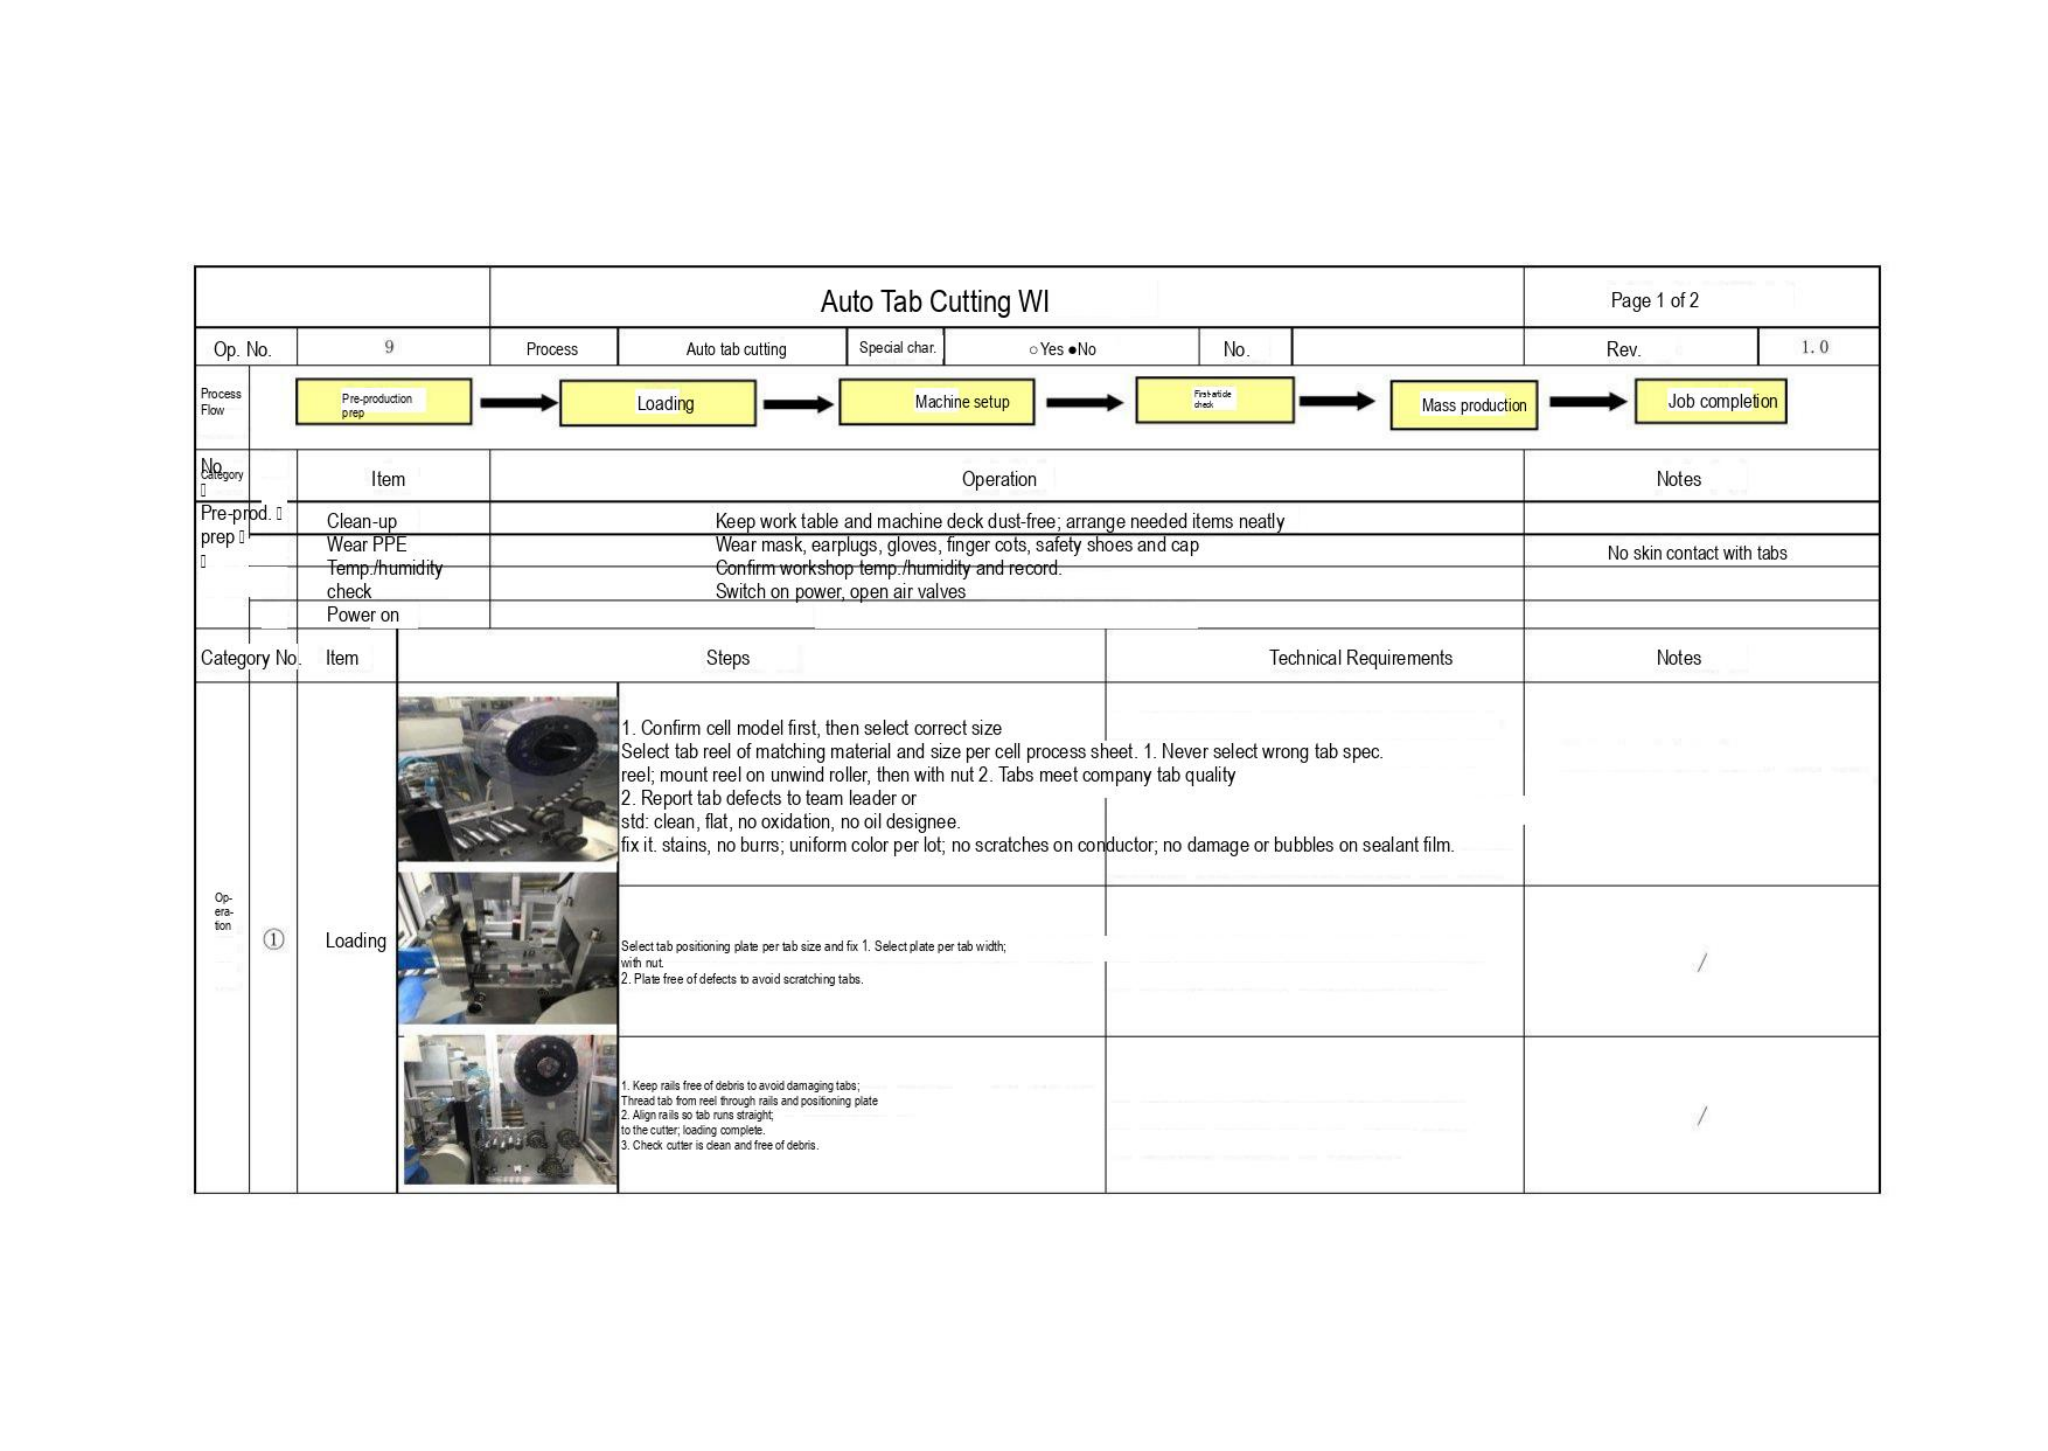# Auto Tab Cutting WI

Page 1 of 2

| Op. No. | 9 | Process | Auto tab cutting | Special char. | ○Yes ●No | No. | | Rev. | 1.0 |
|---|---|---|---|---|---|---|---|---|---|

Process Flow: Pre-production prep → Loading → Machine setup → First article check → Mass production → Job completion

| No. Category | Item | Operation | Notes |
|---|---|---|---|
| Pre-prod. prep | Clean-up | Keep work table and machine deck dust-free; arrange needed items neatly | |
| | Wear PPE | Wear mask, earplugs, gloves, finger cots, safety shoes and cap | No skin contact with tabs |
| | Temp./humidity check | Confirm workshop temp./humidity and record. | |
| | Power on | Switch on power, open air valves | |

| Category | No. | Item | Steps | Technical Requirements | Notes |
|---|---|---|---|---|---|
| Op-era-tion | ① | Loading | 1. Confirm cell model first, then select correct size<br>Select tab reel of matching material and size per cell process sheet. 1. Never select wrong tab spec.<br>reel; mount reel on unwind roller, then with nut 2. Tabs meet company tab quality<br>2. Report tab defects to team leader or<br>std: clean, flat, no oxidation, no oil designee.<br>fix it. stains, no burrs; uniform color per lot; no scratches on conductor; no damage or bubbles on sealant film. | | |
| | | | Select tab positioning plate per tab size and fix 1. Select plate per tab width;<br>with nut.<br>2. Plate free of defects to avoid scratching tabs. | | / |
| | | | 1. Keep rails free of debris to avoid damaging tabs;<br>Thread tab from reel through rails and positioning plate<br>2. Align rails so tab runs straight;<br>to the cutter; loading complete.<br>3. Check cutter is clean and free of debris. | | / |
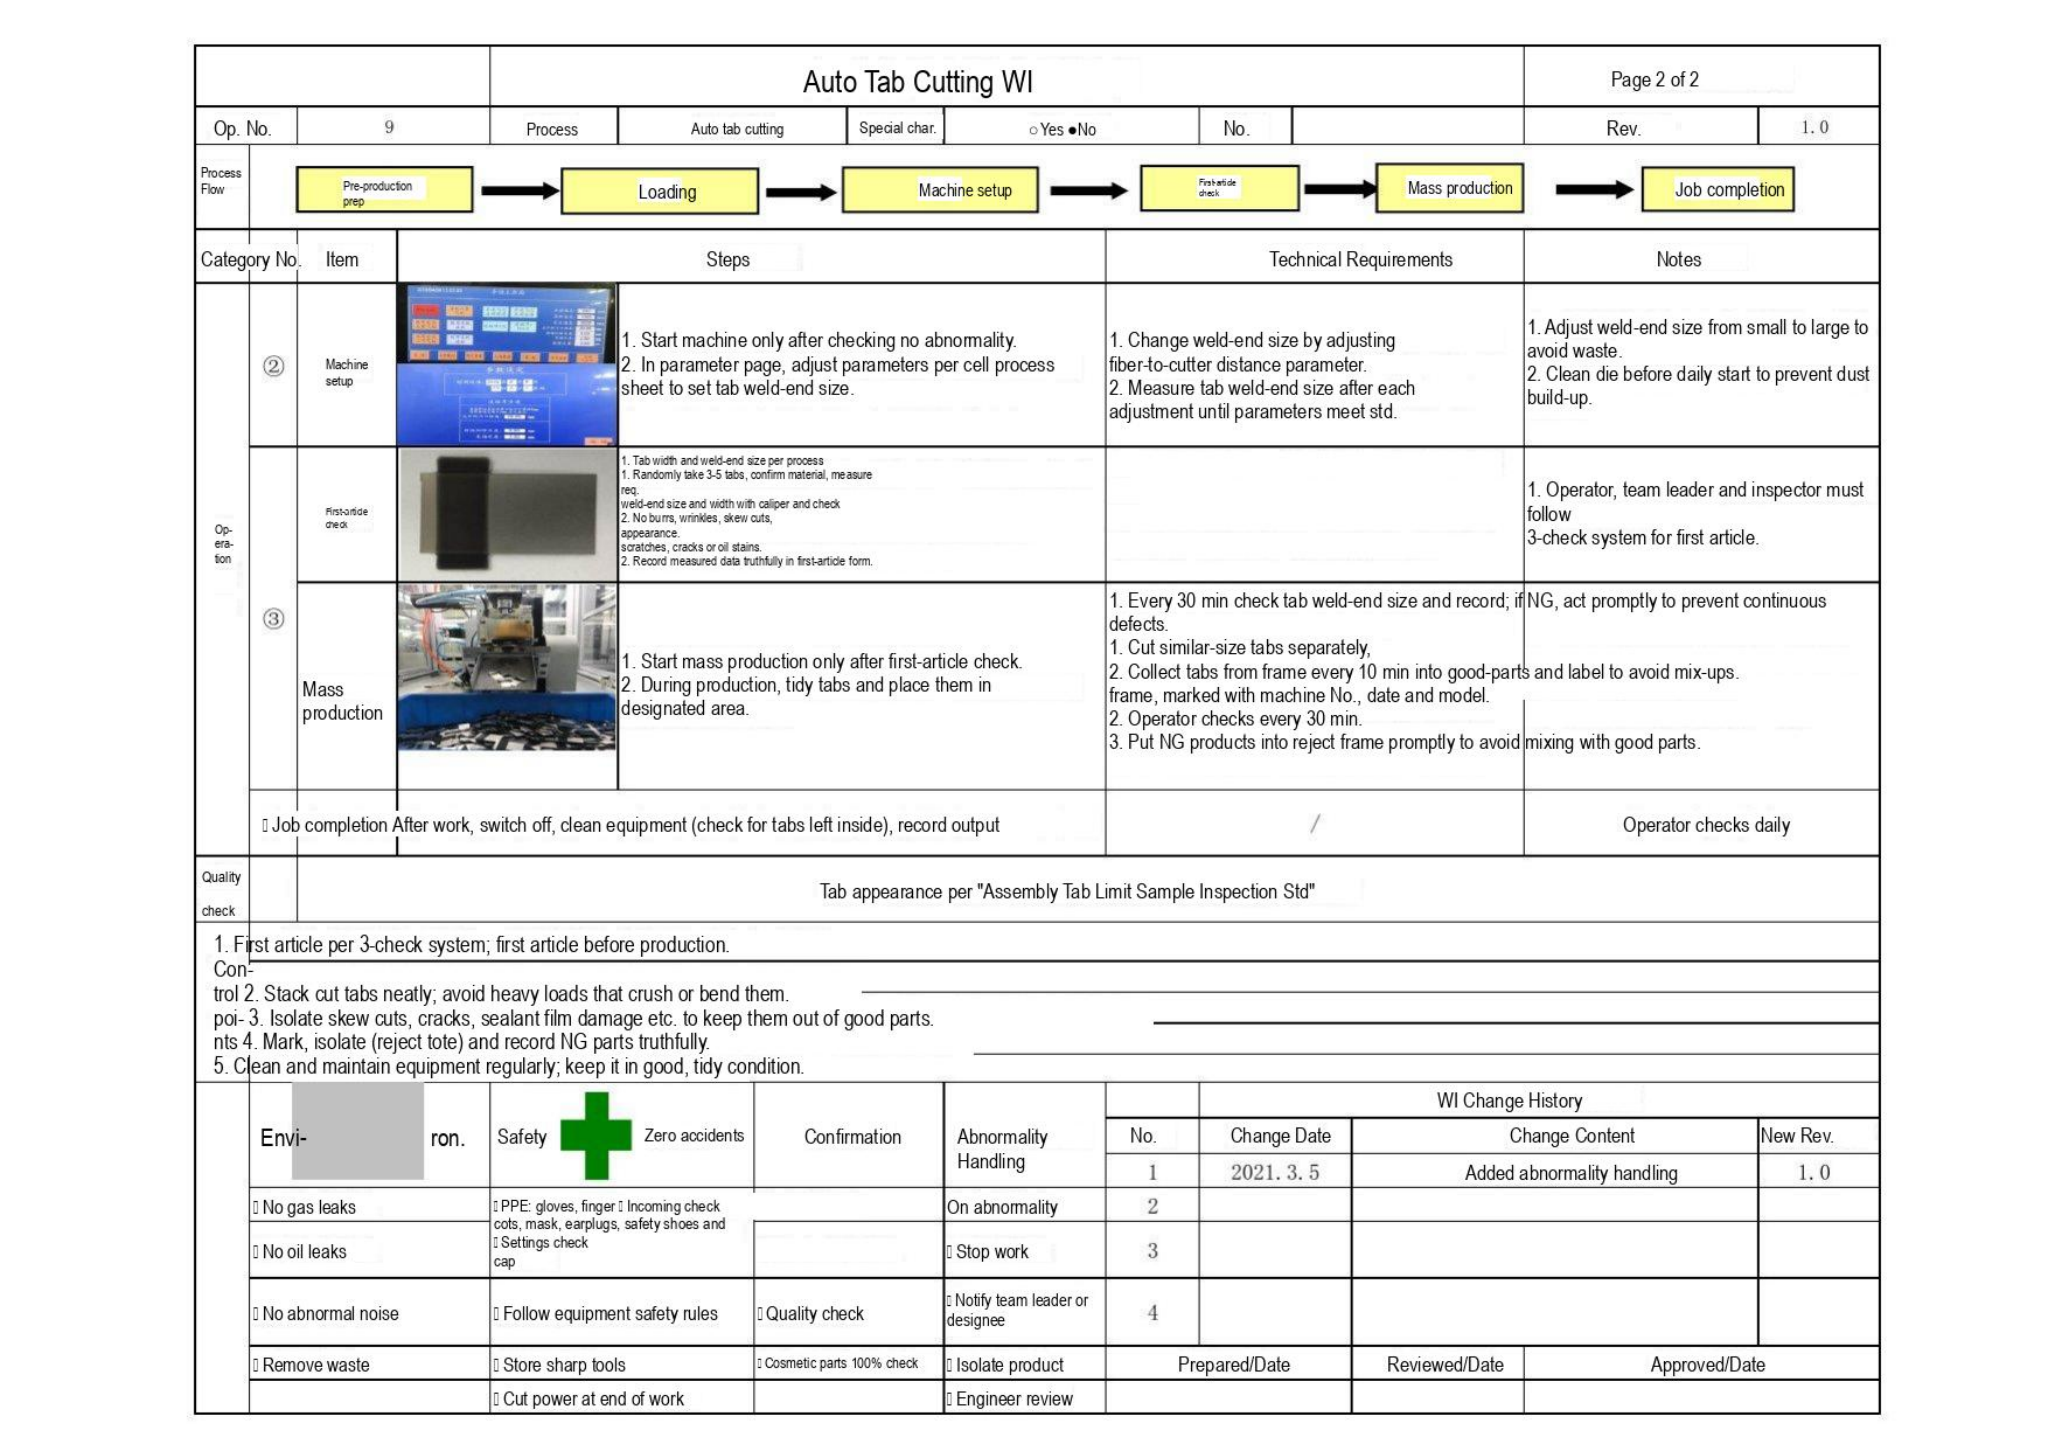# Auto Tab Cutting WI

| | Auto Tab Cutting WI | | | | | | Page 2 of 2 | |
|---|---|---|---|---|---|---|---|---|
| Op. No. | 9 | Process | Auto tab cutting | Special char. | ○Yes ●No | No. | Rev. | 1.0 |

Process Flow: Pre-production prep → Loading → Machine setup → First-article check → Mass production → Job completion

| Category | No. | Item | Steps | Technical Requirements | Notes |
|---|---|---|---|---|---|
| Op-era-tion | ② | Machine setup | 1. Start machine only after checking no abnormality.<br>2. In parameter page, adjust parameters per cell process sheet to set tab weld-end size. | 1. Change weld-end size by adjusting fiber-to-cutter distance parameter.<br>2. Measure tab weld-end size after each adjustment until parameters meet std. | 1. Adjust weld-end size from small to large to avoid waste.<br>2. Clean die before daily start to prevent dust build-up. |
| | | First-article check | 1. Tab width and weld-end size per process<br>1. Randomly take 3-5 tabs, confirm material, measure req.<br>weld-end size and width with caliper and check<br>2. No burrs, wrinkles, skew cuts, appearance.<br>scratches, cracks or oil stains.<br>2. Record measured data truthfully in first-article form. | | 1. Operator, team leader and inspector must follow<br>3-check system for first article. |
| | ③ | Mass production | 1. Start mass production only after first-article check.<br>2. During production, tidy tabs and place them in designated area. | 1. Every 30 min check tab weld-end size and record; if NG, act promptly to prevent continuous defects.<br>1. Cut similar-size tabs separately,<br>2. Collect tabs from frame every 10 min into good-parts and label to avoid mix-ups.<br>frame, marked with machine No., date and model.<br>2. Operator checks every 30 min.<br>3. Put NG products into reject frame promptly to avoid mixing with good parts. | |
| | | □ Job completion | After work, switch off, clean equipment (check for tabs left inside), record output | / | Operator checks daily |
| Quality check | | | Tab appearance per "Assembly Tab Limit Sample Inspection Std" | | |

Con-trol poi-nts
1. First article per 3-check system; first article before production.
2. Stack cut tabs neatly; avoid heavy loads that crush or bend them.
3. Isolate skew cuts, cracks, sealant film damage etc. to keep them out of good parts.
4. Mark, isolate (reject tote) and record NG parts truthfully.
5. Clean and maintain equipment regularly; keep it in good, tidy condition.

| Envi-ron. | Safety Zero accidents | Confirmation | Abnormality Handling | No. | Change Date | Change Content | New Rev. |
|---|---|---|---|---|---|---|---|
| | | | | 1 | 2021.3.5 | Added abnormality handling | 1.0 |
| □ No gas leaks | □ PPE: gloves, finger cots, mask, earplugs, safety shoes and cap | □ Incoming check<br>□ Settings check | On abnormality | 2 | | | |
| □ No oil leaks | | | □ Stop work | 3 | | | |
| □ No abnormal noise | □ Follow equipment safety rules | □ Quality check | □ Notify team leader or designee | 4 | | | |
| □ Remove waste | □ Store sharp tools | □ Cosmetic parts 100% check | □ Isolate product | Prepared/Date | Reviewed/Date | Approved/Date | |
| | □ Cut power at end of work | | □ Engineer review | | | | |

WI Change History